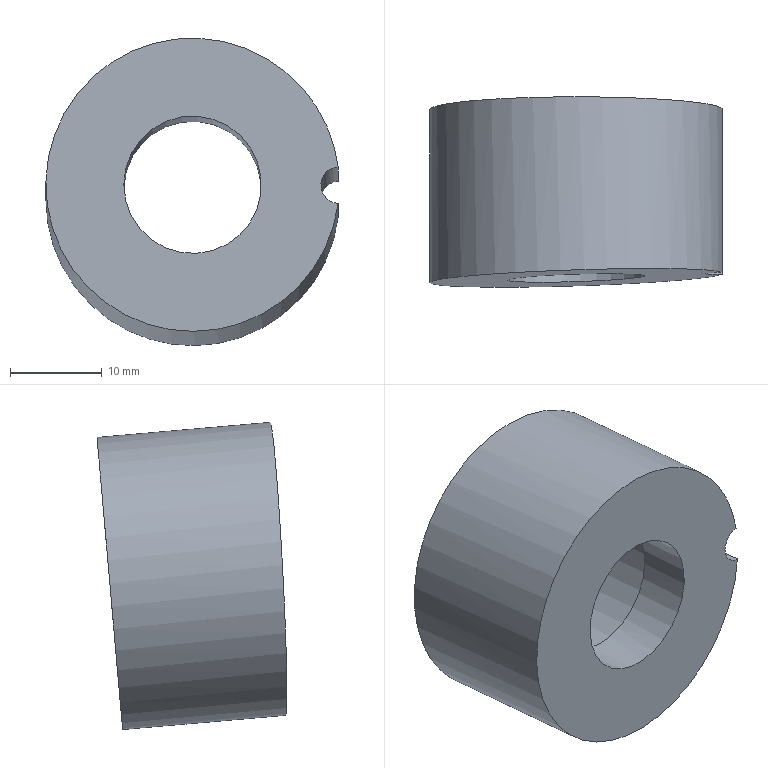Part | NX | features EKSD 32-20-18.00 2 | 1 solid | 7 faces | box 31.875 x 20.717 x 33.529 mm | volume 9556 mm3 | cylinder 4 | plane 3 | commonest cylinder face diameters 4 x1 15 x1 20.6 x1 32 x1
STEP:
#1=CARTESIAN_POINT('',(-307.101,-42.459,-36.691));
#2=VERTEX_POINT('',#1);
#3=CARTESIAN_POINT('',(-307.101,-42.807,-40.668));
#4=VERTEX_POINT('',#3);
#5=CARTESIAN_POINT('',(-306.976,-42.633,-38.68));
#6=DIRECTION('',(0.,-0.9962,0.08716));
#7=DIRECTION('',(-1.,0.,0.));
#8=AXIS2_PLACEMENT_3D('',#5,#6,#7);
#9=CIRCLE('',#8,2.);
#10=EDGE_CURVE('',#2,#4,#9,.T.);
#11=ORIENTED_EDGE('',*,*,#10,.T.);
#12=CARTESIAN_POINT('',(-322.976,-42.633,-38.68));
#13=DIRECTION('',(0.,-0.9962,0.08716));
#14=DIRECTION('',(-1.,0.,0.));
#15=AXIS2_PLACEMENT_3D('',#12,#13,#14);
#16=CIRCLE('',#15,16.);
#17=EDGE_CURVE('',#2,#4,#16,.T.);
#18=ORIENTED_EDGE('',*,*,#17,.F.);
#19=EDGE_LOOP('',(#11,#18));
#20=FACE_BOUND('',#19,.T.);
#21=CARTESIAN_POINT('',(-312.676,-42.633,-38.68));
#22=VERTEX_POINT('',#21);
#23=CARTESIAN_POINT('',(-322.976,-42.633,-38.68));
#24=DIRECTION('',(0.,0.9962,-0.08716));
#25=DIRECTION('',(1.,0.,0.));
#26=AXIS2_PLACEMENT_3D('',#23,#24,#25);
#27=CIRCLE('',#26,10.3);
#28=EDGE_CURVE('',#22,#22,#27,.T.);
#29=ORIENTED_EDGE('',*,*,#28,.F.);
#30=EDGE_LOOP('',(#29));
#31=FACE_BOUND('',#30,.T.);
#32=CARTESIAN_POINT('',(-322.976,-42.633,-38.68));
#33=DIRECTION('',(0.,0.9962,-0.08716));
#34=DIRECTION('',(1.,0.,0.));
#35=AXIS2_PLACEMENT_3D('',#32,#33,#34);
#36=PLANE('',#35);
#37=ADVANCED_FACE('',(#20,#31),#36,.T.);
#38=CARTESIAN_POINT('',(-307.101,-60.551,-39.116));
#39=VERTEX_POINT('',#38);
#40=CARTESIAN_POINT('',(-307.101,-60.339,-35.127));
#41=VERTEX_POINT('',#40);
#42=CARTESIAN_POINT('',(-306.976,-60.441,-37.122));
#43=DIRECTION('',(-0.03252,0.9981,-0.05307));
#44=DIRECTION('',(0.6892,-0.01607,-0.7244));
#45=AXIS2_PLACEMENT_3D('',#42,#43,#44);
#46=ELLIPSE('',#45,2.002,2.);
#47=EDGE_CURVE('',#39,#41,#46,.T.);
#48=ORIENTED_EDGE('',*,*,#47,.T.);
#49=CARTESIAN_POINT('',(-322.976,-60.96,-37.076));
#50=DIRECTION('',(-0.03252,0.9981,-0.05307));
#51=DIRECTION('',(0.6892,-0.01607,-0.7244));
#52=AXIS2_PLACEMENT_3D('',#49,#50,#51);
#53=ELLIPSE('',#52,16.018,16.);
#54=EDGE_CURVE('',#39,#41,#53,.T.);
#55=ORIENTED_EDGE('',*,*,#54,.F.);
#56=EDGE_LOOP('',(#48,#55));
#57=FACE_BOUND('',#56,.T.);
#58=CARTESIAN_POINT('',(-317.802,-61.081,-42.516));
#59=VERTEX_POINT('',#58);
#60=CARTESIAN_POINT('',(-322.976,-60.96,-37.076));
#61=DIRECTION('',(-0.03252,0.9981,-0.05307));
#62=DIRECTION('',(0.6892,-0.01607,-0.7244));
#63=AXIS2_PLACEMENT_3D('',#60,#61,#62);
#64=ELLIPSE('',#63,7.508,7.5);
#65=EDGE_CURVE('',#59,#59,#64,.F.);
#66=ORIENTED_EDGE('',*,*,#65,.F.);
#67=EDGE_LOOP('',(#66));
#68=FACE_BOUND('',#67,.T.);
#69=CARTESIAN_POINT('',(-422.194,-57.948,80.353));
#70=DIRECTION('',(-0.03252,0.9981,-0.05307));
#71=DIRECTION('',(0.05223,-0.05133,-0.9973));
#72=AXIS2_PLACEMENT_3D('',#69,#70,#71);
#73=PLANE('',#72);
#74=ADVANCED_FACE('',(#57,#68),#73,.F.);
#75=CARTESIAN_POINT('',(-307.101,-52.769,-39.797));
#76=DIRECTION('',(0.,0.9962,-0.08716));
#77=VECTOR('',#76,1000.);
#78=LINE('',#75,#77);
#79=EDGE_CURVE('',#39,#4,#78,.T.);
#80=ORIENTED_EDGE('',*,*,#79,.F.);
#81=ORIENTED_EDGE('',*,*,#54,.T.);
#82=CARTESIAN_POINT('',(-307.101,-52.421,-35.82));
#83=DIRECTION('',(0.,0.9962,-0.08716));
#84=VECTOR('',#83,1000.);
#85=LINE('',#82,#84);
#86=EDGE_CURVE('',#2,#41,#85,.F.);
#87=ORIENTED_EDGE('',*,*,#86,.F.);
#88=ORIENTED_EDGE('',*,*,#17,.T.);
#89=EDGE_LOOP('',(#80,#81,#87,#88));
#90=FACE_BOUND('',#89,.T.);
#91=CARTESIAN_POINT('',(-322.976,-62.557,-36.937));
#92=DIRECTION('',(0.,0.9962,-0.08716));
#93=DIRECTION('',(1.,0.,0.));
#94=AXIS2_PLACEMENT_3D('',#91,#92,#93);
#95=CYLINDRICAL_SURFACE('',#94,16.);
#96=ADVANCED_FACE('',(#90),#95,.T.);
#97=CARTESIAN_POINT('',(-322.976,-55.241,-45.105));
#98=VERTEX_POINT('',#97);
#99=CARTESIAN_POINT('',(-322.976,-54.587,-37.634));
#100=DIRECTION('',(0.,-0.9962,0.08716));
#101=DIRECTION('',(0.,-0.08716,-0.9962));
#102=AXIS2_PLACEMENT_3D('',#99,#100,#101);
#103=CIRCLE('',#102,7.5);
#104=EDGE_CURVE('',#98,#98,#103,.F.);
#105=ORIENTED_EDGE('',*,*,#104,.T.);
#106=EDGE_LOOP('',(#105));
#107=FACE_BOUND('',#106,.T.);
#108=ORIENTED_EDGE('',*,*,#65,.T.);
#109=EDGE_LOOP('',(#108));
#110=FACE_BOUND('',#109,.T.);
#111=CARTESIAN_POINT('',(-322.976,-63.553,-36.85));
#112=DIRECTION('',(0.,0.9962,-0.08716));
#113=DIRECTION('',(1.,0.,0.));
#114=AXIS2_PLACEMENT_3D('',#111,#112,#113);
#115=CYLINDRICAL_SURFACE('',#114,7.5);
#116=ADVANCED_FACE('',(#107,#110),#115,.F.);
#117=CARTESIAN_POINT('',(-312.676,-54.587,-37.634));
#118=VERTEX_POINT('',#117);
#119=CARTESIAN_POINT('',(-322.976,-54.587,-37.634));
#120=DIRECTION('',(0.,0.9962,-0.08716));
#121=DIRECTION('',(1.,0.,0.));
#122=AXIS2_PLACEMENT_3D('',#119,#120,#121);
#123=CIRCLE('',#122,10.3);
#124=EDGE_CURVE('',#118,#118,#123,.T.);
#125=ORIENTED_EDGE('',*,*,#124,.T.);
#126=EDGE_LOOP('',(#125));
#127=FACE_BOUND('',#126,.T.);
#128=ORIENTED_EDGE('',*,*,#104,.F.);
#129=EDGE_LOOP('',(#128));
#130=FACE_BOUND('',#129,.T.);
#131=CARTESIAN_POINT('',(-322.976,-54.587,-37.634));
#132=DIRECTION('',(0.,-0.9962,0.08716));
#133=DIRECTION('',(-1.,0.,0.));
#134=AXIS2_PLACEMENT_3D('',#131,#132,#133);
#135=PLANE('',#134);
#136=ADVANCED_FACE('',(#127,#130),#135,.F.);
#137=ORIENTED_EDGE('',*,*,#28,.T.);
#138=EDGE_LOOP('',(#137));
#139=FACE_BOUND('',#138,.T.);
#140=ORIENTED_EDGE('',*,*,#124,.F.);
#141=EDGE_LOOP('',(#140));
#142=FACE_BOUND('',#141,.T.);
#143=CARTESIAN_POINT('',(-322.976,-54.587,-37.634));
#144=DIRECTION('',(0.,0.9962,-0.08716));
#145=DIRECTION('',(1.,0.,0.));
#146=AXIS2_PLACEMENT_3D('',#143,#144,#145);
#147=CYLINDRICAL_SURFACE('',#146,10.3);
#148=ADVANCED_FACE('',(#139,#142),#147,.F.);
#149=ORIENTED_EDGE('',*,*,#79,.T.);
#150=ORIENTED_EDGE('',*,*,#10,.F.);
#151=ORIENTED_EDGE('',*,*,#86,.T.);
#152=ORIENTED_EDGE('',*,*,#47,.F.);
#153=EDGE_LOOP('',(#149,#150,#151,#152));
#154=FACE_BOUND('',#153,.T.);
#155=CARTESIAN_POINT('',(-306.976,-62.557,-36.937));
#156=DIRECTION('',(0.,0.9962,-0.08716));
#157=DIRECTION('',(1.,0.,0.));
#158=AXIS2_PLACEMENT_3D('',#155,#156,#157);
#159=CYLINDRICAL_SURFACE('',#158,2.);
#160=ADVANCED_FACE('',(#154),#159,.F.);
#161=CLOSED_SHELL('',(#37,#74,#96,#116,#136,#148,#160));
#162=MANIFOLD_SOLID_BREP('',#161);
#163=(LENGTH_UNIT()NAMED_UNIT(*)SI_UNIT(.MILLI.,.METRE.));
#164=UNCERTAINTY_MEASURE_WITH_UNIT(LENGTH_MEASURE(0.00001),#163,'','');
#165=(NAMED_UNIT(*)PLANE_ANGLE_UNIT()SI_UNIT($,.RADIAN.));
#166=(NAMED_UNIT(*)SI_UNIT($,.STERADIAN.)SOLID_ANGLE_UNIT());
#167=(GEOMETRIC_REPRESENTATION_CONTEXT(3)GLOBAL_UNCERTAINTY_ASSIGNED_CONTEXT((#164))GLOBAL_UNIT_ASSIGNED_CONTEXT((#163,#165,#166))REPRESENTATION_CONTEXT('',''));
#168=ADVANCED_BREP_SHAPE_REPRESENTATION('',(#162),#167);